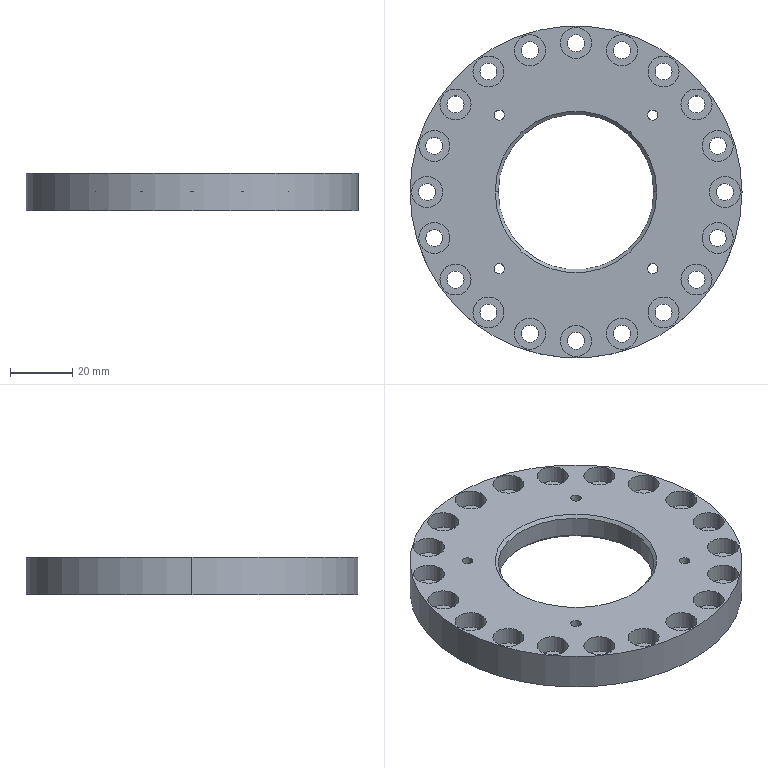Part | SolidWorks | features CirPattern 2, HoleWzd 2, Chamfer 1, Extrusion 1, ICE 1 | 1 solid | 129 faces | box 107 x 107 x 12 mm | volume 66155 mm3 | cylinder 97 | plane 23 | cone 9 | commonest cylinder face diameters 5.5 x40 10 x40 3.3 x8 67.1 x5 50.1 x2 107 x2